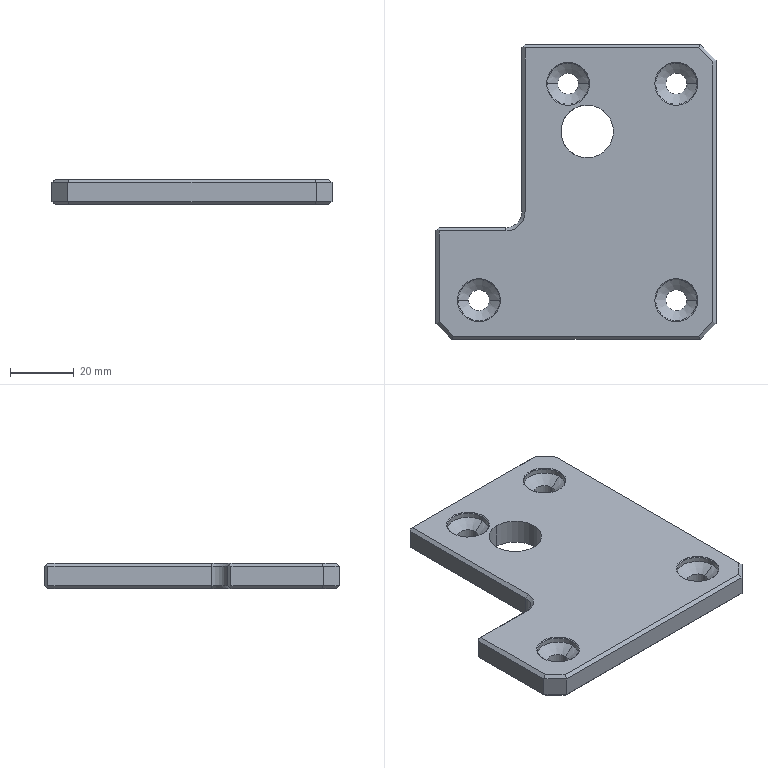Part | Creo | 1 solid | 68 faces | box 88 x 92.5 x 8 mm | volume 48143 mm3 | plane 31 | cylinder 19 | cone 18 | commonest cylinder face diameters 6.6 x8 13 x8 16.5 x2 10 x1